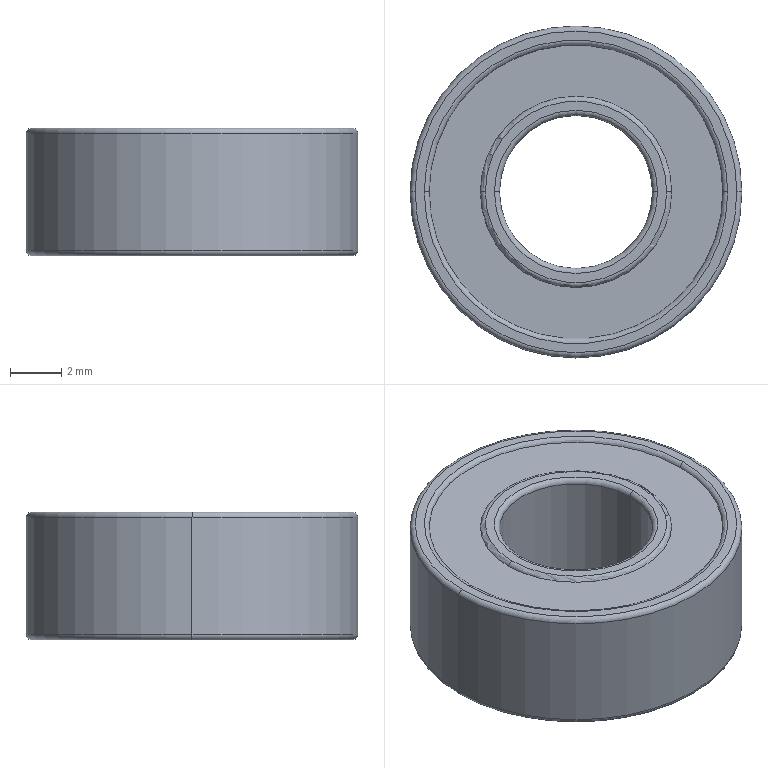Part | NX | features BREP 1 | 1 solid | 26 faces | box 13 x 13 x 5 mm | volume 502.459 mm3 | torus 16 | plane 6 | cylinder 4 | commonest cylinder face diameters 6 x2 13 x2
STEP:
#1=CARTESIAN_POINT('',(3.,0.,-0.2));
#2=VERTEX_POINT('',#1);
#3=CARTESIAN_POINT('',(3.2,0.,0.));
#4=VERTEX_POINT('',#3);
#5=CARTESIAN_POINT('',(3.2,0.,-0.2));
#6=DIRECTION('',(0.,1.,0.));
#7=DIRECTION('',(-1.,0.,0.));
#8=AXIS2_PLACEMENT_3D('',#5,#6,#7);
#9=CIRCLE('',#8,0.2);
#10=EDGE_CURVE('',#2,#4,#9,.T.);
#11=ORIENTED_EDGE('',*,*,#10,.F.);
#12=CARTESIAN_POINT('',(-3.,0.,-0.2));
#13=VERTEX_POINT('',#12);
#14=CARTESIAN_POINT('',(0.,0.,-0.2));
#15=DIRECTION('',(0.,0.,1.));
#16=DIRECTION('',(-1.,0.,0.));
#17=AXIS2_PLACEMENT_3D('',#14,#15,#16);
#18=CIRCLE('',#17,3.);
#19=EDGE_CURVE('',#13,#2,#18,.T.);
#20=ORIENTED_EDGE('',*,*,#19,.F.);
#21=CARTESIAN_POINT('',(-3.2,0.,0.));
#22=VERTEX_POINT('',#21);
#23=CARTESIAN_POINT('',(-3.2,0.,-0.2));
#24=DIRECTION('',(0.,-1.,0.));
#25=DIRECTION('',(0.,0.,-1.));
#26=AXIS2_PLACEMENT_3D('',#23,#24,#25);
#27=CIRCLE('',#26,0.2);
#28=EDGE_CURVE('',#13,#22,#27,.T.);
#29=ORIENTED_EDGE('',*,*,#28,.T.);
#30=CARTESIAN_POINT('',(0.,0.,0.));
#31=DIRECTION('',(0.,0.,-1.));
#32=DIRECTION('',(-1.,0.,0.));
#33=AXIS2_PLACEMENT_3D('',#30,#31,#32);
#34=CIRCLE('',#33,3.2);
#35=EDGE_CURVE('',#4,#22,#34,.T.);
#36=ORIENTED_EDGE('',*,*,#35,.F.);
#37=EDGE_LOOP('',(#11,#20,#29,#36));
#38=FACE_BOUND('',#37,.T.);
#39=CARTESIAN_POINT('',(0.,0.,-0.2));
#40=DIRECTION('',(0.,0.,-1.));
#41=DIRECTION('',(-1.,0.,0.));
#42=AXIS2_PLACEMENT_3D('',#39,#40,#41);
#43=TOROIDAL_SURFACE('',#42,3.2,0.2);
#44=ADVANCED_FACE('',(#38),#43,.T.);
#45=CARTESIAN_POINT('',(5.75,0.,-0.15));
#46=VERTEX_POINT('',#45);
#47=CARTESIAN_POINT('',(5.944,0.,0.));
#48=VERTEX_POINT('',#47);
#49=CARTESIAN_POINT('',(5.944,0.,-0.2));
#50=DIRECTION('',(0.,1.,0.));
#51=DIRECTION('',(-1.,0.,0.));
#52=AXIS2_PLACEMENT_3D('',#49,#50,#51);
#53=CIRCLE('',#52,0.2);
#54=EDGE_CURVE('',#46,#48,#53,.T.);
#55=ORIENTED_EDGE('',*,*,#54,.F.);
#56=CARTESIAN_POINT('',(-5.75,0.,-0.15));
#57=VERTEX_POINT('',#56);
#58=CARTESIAN_POINT('',(0.,0.,-0.15));
#59=DIRECTION('',(0.,0.,1.));
#60=DIRECTION('',(1.,0.,0.));
#61=AXIS2_PLACEMENT_3D('',#58,#59,#60);
#62=CIRCLE('',#61,5.75);
#63=EDGE_CURVE('',#57,#46,#62,.T.);
#64=ORIENTED_EDGE('',*,*,#63,.F.);
#65=CARTESIAN_POINT('',(-5.944,0.,0.));
#66=VERTEX_POINT('',#65);
#67=CARTESIAN_POINT('',(-5.944,0.,-0.2));
#68=DIRECTION('',(0.,-1.,0.));
#69=DIRECTION('',(0.,0.,-1.));
#70=AXIS2_PLACEMENT_3D('',#67,#68,#69);
#71=CIRCLE('',#70,0.2);
#72=EDGE_CURVE('',#57,#66,#71,.T.);
#73=ORIENTED_EDGE('',*,*,#72,.T.);
#74=CARTESIAN_POINT('',(0.,0.,0.));
#75=DIRECTION('',(0.,0.,-1.));
#76=DIRECTION('',(-1.,0.,0.));
#77=AXIS2_PLACEMENT_3D('',#74,#75,#76);
#78=CIRCLE('',#77,5.944);
#79=EDGE_CURVE('',#48,#66,#78,.T.);
#80=ORIENTED_EDGE('',*,*,#79,.F.);
#81=EDGE_LOOP('',(#55,#64,#73,#80));
#82=FACE_BOUND('',#81,.T.);
#83=CARTESIAN_POINT('',(0.,0.,-0.2));
#84=DIRECTION('',(0.,0.,-1.));
#85=DIRECTION('',(-1.,0.,0.));
#86=AXIS2_PLACEMENT_3D('',#83,#84,#85);
#87=TOROIDAL_SURFACE('',#86,5.944,0.2);
#88=ADVANCED_FACE('',(#82),#87,.T.);
#89=CARTESIAN_POINT('',(-3.556,0.,0.));
#90=VERTEX_POINT('',#89);
#91=CARTESIAN_POINT('',(-3.75,0.,-0.15));
#92=VERTEX_POINT('',#91);
#93=CARTESIAN_POINT('',(-3.556,0.,-0.2));
#94=DIRECTION('',(0.,1.,0.));
#95=DIRECTION('',(-1.,0.,0.));
#96=AXIS2_PLACEMENT_3D('',#93,#94,#95);
#97=CIRCLE('',#96,0.2);
#98=EDGE_CURVE('',#90,#92,#97,.F.);
#99=ORIENTED_EDGE('',*,*,#98,.T.);
#100=CARTESIAN_POINT('',(3.75,0.,-0.15));
#101=VERTEX_POINT('',#100);
#102=CARTESIAN_POINT('',(0.,0.,-0.15));
#103=DIRECTION('',(0.,0.,1.));
#104=DIRECTION('',(1.,0.,0.));
#105=AXIS2_PLACEMENT_3D('',#102,#103,#104);
#106=CIRCLE('',#105,3.75);
#107=EDGE_CURVE('',#92,#101,#106,.T.);
#108=ORIENTED_EDGE('',*,*,#107,.T.);
#109=CARTESIAN_POINT('',(3.556,0.,0.));
#110=VERTEX_POINT('',#109);
#111=CARTESIAN_POINT('',(3.556,0.,-0.2));
#112=DIRECTION('',(0.,-1.,0.));
#113=DIRECTION('',(0.,0.,-1.));
#114=AXIS2_PLACEMENT_3D('',#111,#112,#113);
#115=CIRCLE('',#114,0.2);
#116=EDGE_CURVE('',#110,#101,#115,.F.);
#117=ORIENTED_EDGE('',*,*,#116,.F.);
#118=CARTESIAN_POINT('',(0.,0.,0.));
#119=DIRECTION('',(0.,0.,1.));
#120=DIRECTION('',(-1.,0.,0.));
#121=AXIS2_PLACEMENT_3D('',#118,#119,#120);
#122=CIRCLE('',#121,3.556);
#123=EDGE_CURVE('',#90,#110,#122,.T.);
#124=ORIENTED_EDGE('',*,*,#123,.F.);
#125=EDGE_LOOP('',(#99,#108,#117,#124));
#126=FACE_BOUND('',#125,.T.);
#127=CARTESIAN_POINT('',(0.,0.,-0.2));
#128=DIRECTION('',(0.,0.,1.));
#129=DIRECTION('',(1.,0.,0.));
#130=AXIS2_PLACEMENT_3D('',#127,#128,#129);
#131=TOROIDAL_SURFACE('',#130,3.556,0.2);
#132=ADVANCED_FACE('',(#126),#131,.T.);
#133=CARTESIAN_POINT('',(6.3,0.,0.));
#134=VERTEX_POINT('',#133);
#135=CARTESIAN_POINT('',(6.5,0.,-0.2));
#136=VERTEX_POINT('',#135);
#137=CARTESIAN_POINT('',(6.3,0.,-0.2));
#138=DIRECTION('',(0.,1.,0.));
#139=DIRECTION('',(-1.,0.,0.));
#140=AXIS2_PLACEMENT_3D('',#137,#138,#139);
#141=CIRCLE('',#140,0.2);
#142=EDGE_CURVE('',#134,#136,#141,.T.);
#143=ORIENTED_EDGE('',*,*,#142,.F.);
#144=CARTESIAN_POINT('',(-6.3,0.,0.));
#145=VERTEX_POINT('',#144);
#146=CARTESIAN_POINT('',(0.,0.,0.));
#147=DIRECTION('',(0.,0.,1.));
#148=DIRECTION('',(-1.,0.,0.));
#149=AXIS2_PLACEMENT_3D('',#146,#147,#148);
#150=CIRCLE('',#149,6.3);
#151=EDGE_CURVE('',#145,#134,#150,.T.);
#152=ORIENTED_EDGE('',*,*,#151,.F.);
#153=CARTESIAN_POINT('',(-6.5,0.,-0.2));
#154=VERTEX_POINT('',#153);
#155=CARTESIAN_POINT('',(-6.3,0.,-0.2));
#156=DIRECTION('',(0.,-1.,0.));
#157=DIRECTION('',(0.,0.,-1.));
#158=AXIS2_PLACEMENT_3D('',#155,#156,#157);
#159=CIRCLE('',#158,0.2);
#160=EDGE_CURVE('',#145,#154,#159,.T.);
#161=ORIENTED_EDGE('',*,*,#160,.T.);
#162=CARTESIAN_POINT('',(0.,0.,-0.2));
#163=DIRECTION('',(0.,0.,-1.));
#164=DIRECTION('',(-1.,0.,0.));
#165=AXIS2_PLACEMENT_3D('',#162,#163,#164);
#166=CIRCLE('',#165,6.5);
#167=EDGE_CURVE('',#136,#154,#166,.T.);
#168=ORIENTED_EDGE('',*,*,#167,.F.);
#169=EDGE_LOOP('',(#143,#152,#161,#168));
#170=FACE_BOUND('',#169,.T.);
#171=CARTESIAN_POINT('',(0.,0.,-0.2));
#172=DIRECTION('',(0.,0.,-1.));
#173=DIRECTION('',(-1.,0.,0.));
#174=AXIS2_PLACEMENT_3D('',#171,#172,#173);
#175=TOROIDAL_SURFACE('',#174,6.3,0.2);
#176=ADVANCED_FACE('',(#170),#175,.T.);
#177=CARTESIAN_POINT('',(-6.5,0.,-4.8));
#178=VERTEX_POINT('',#177);
#179=CARTESIAN_POINT('',(-6.3,0.,-5.));
#180=VERTEX_POINT('',#179);
#181=CARTESIAN_POINT('',(-6.3,0.,-4.8));
#182=DIRECTION('',(0.,1.,0.));
#183=DIRECTION('',(-1.,0.,0.));
#184=AXIS2_PLACEMENT_3D('',#181,#182,#183);
#185=CIRCLE('',#184,0.2);
#186=EDGE_CURVE('',#178,#180,#185,.F.);
#187=ORIENTED_EDGE('',*,*,#186,.T.);
#188=CARTESIAN_POINT('',(6.3,0.,-5.));
#189=VERTEX_POINT('',#188);
#190=CARTESIAN_POINT('',(0.,0.,-5.));
#191=DIRECTION('',(0.,0.,-1.));
#192=DIRECTION('',(1.,0.,0.));
#193=AXIS2_PLACEMENT_3D('',#190,#191,#192);
#194=CIRCLE('',#193,6.3);
#195=EDGE_CURVE('',#189,#180,#194,.T.);
#196=ORIENTED_EDGE('',*,*,#195,.F.);
#197=CARTESIAN_POINT('',(6.5,0.,-4.8));
#198=VERTEX_POINT('',#197);
#199=CARTESIAN_POINT('',(6.3,0.,-4.8));
#200=DIRECTION('',(0.,-1.,0.));
#201=DIRECTION('',(0.,0.,-1.));
#202=AXIS2_PLACEMENT_3D('',#199,#200,#201);
#203=CIRCLE('',#202,0.2);
#204=EDGE_CURVE('',#198,#189,#203,.F.);
#205=ORIENTED_EDGE('',*,*,#204,.F.);
#206=CARTESIAN_POINT('',(0.,0.,-4.8));
#207=DIRECTION('',(0.,0.,1.));
#208=DIRECTION('',(1.,0.,0.));
#209=AXIS2_PLACEMENT_3D('',#206,#207,#208);
#210=CIRCLE('',#209,6.5);
#211=EDGE_CURVE('',#178,#198,#210,.T.);
#212=ORIENTED_EDGE('',*,*,#211,.F.);
#213=EDGE_LOOP('',(#187,#196,#205,#212));
#214=FACE_BOUND('',#213,.T.);
#215=CARTESIAN_POINT('',(0.,0.,-4.8));
#216=DIRECTION('',(0.,0.,1.));
#217=DIRECTION('',(1.,0.,0.));
#218=AXIS2_PLACEMENT_3D('',#215,#216,#217);
#219=TOROIDAL_SURFACE('',#218,6.3,0.2);
#220=ADVANCED_FACE('',(#214),#219,.T.);
#221=CARTESIAN_POINT('',(-5.944,0.,-5.));
#222=VERTEX_POINT('',#221);
#223=CARTESIAN_POINT('',(-5.75,0.,-4.85));
#224=VERTEX_POINT('',#223);
#225=CARTESIAN_POINT('',(-5.944,0.,-4.8));
#226=DIRECTION('',(0.,1.,0.));
#227=DIRECTION('',(-1.,0.,0.));
#228=AXIS2_PLACEMENT_3D('',#225,#226,#227);
#229=CIRCLE('',#228,0.2);
#230=EDGE_CURVE('',#222,#224,#229,.F.);
#231=ORIENTED_EDGE('',*,*,#230,.T.);
#232=CARTESIAN_POINT('',(5.75,0.,-4.85));
#233=VERTEX_POINT('',#232);
#234=CARTESIAN_POINT('',(0.,0.,-4.85));
#235=DIRECTION('',(0.,0.,1.));
#236=DIRECTION('',(1.,0.,0.));
#237=AXIS2_PLACEMENT_3D('',#234,#235,#236);
#238=CIRCLE('',#237,5.75);
#239=EDGE_CURVE('',#224,#233,#238,.T.);
#240=ORIENTED_EDGE('',*,*,#239,.T.);
#241=CARTESIAN_POINT('',(5.944,0.,-5.));
#242=VERTEX_POINT('',#241);
#243=CARTESIAN_POINT('',(5.944,0.,-4.8));
#244=DIRECTION('',(0.,-1.,0.));
#245=DIRECTION('',(0.,0.,-1.));
#246=AXIS2_PLACEMENT_3D('',#243,#244,#245);
#247=CIRCLE('',#246,0.2);
#248=EDGE_CURVE('',#242,#233,#247,.F.);
#249=ORIENTED_EDGE('',*,*,#248,.F.);
#250=CARTESIAN_POINT('',(0.,0.,-5.));
#251=DIRECTION('',(0.,0.,1.));
#252=DIRECTION('',(1.,0.,0.));
#253=AXIS2_PLACEMENT_3D('',#250,#251,#252);
#254=CIRCLE('',#253,5.944);
#255=EDGE_CURVE('',#222,#242,#254,.T.);
#256=ORIENTED_EDGE('',*,*,#255,.F.);
#257=EDGE_LOOP('',(#231,#240,#249,#256));
#258=FACE_BOUND('',#257,.T.);
#259=CARTESIAN_POINT('',(0.,0.,-4.8));
#260=DIRECTION('',(0.,0.,1.));
#261=DIRECTION('',(1.,0.,0.));
#262=AXIS2_PLACEMENT_3D('',#259,#260,#261);
#263=TOROIDAL_SURFACE('',#262,5.944,0.2);
#264=ADVANCED_FACE('',(#258),#263,.T.);
#265=CARTESIAN_POINT('',(3.75,0.,-4.85));
#266=VERTEX_POINT('',#265);
#267=CARTESIAN_POINT('',(3.556,0.,-5.));
#268=VERTEX_POINT('',#267);
#269=CARTESIAN_POINT('',(3.556,0.,-4.8));
#270=DIRECTION('',(0.,1.,0.));
#271=DIRECTION('',(-1.,0.,0.));
#272=AXIS2_PLACEMENT_3D('',#269,#270,#271);
#273=CIRCLE('',#272,0.2);
#274=EDGE_CURVE('',#266,#268,#273,.T.);
#275=ORIENTED_EDGE('',*,*,#274,.F.);
#276=CARTESIAN_POINT('',(-3.75,0.,-4.85));
#277=VERTEX_POINT('',#276);
#278=CARTESIAN_POINT('',(0.,0.,-4.85));
#279=DIRECTION('',(0.,0.,1.));
#280=DIRECTION('',(1.,0.,0.));
#281=AXIS2_PLACEMENT_3D('',#278,#279,#280);
#282=CIRCLE('',#281,3.75);
#283=EDGE_CURVE('',#277,#266,#282,.T.);
#284=ORIENTED_EDGE('',*,*,#283,.F.);
#285=CARTESIAN_POINT('',(-3.556,0.,-5.));
#286=VERTEX_POINT('',#285);
#287=CARTESIAN_POINT('',(-3.556,0.,-4.8));
#288=DIRECTION('',(0.,-1.,0.));
#289=DIRECTION('',(0.,0.,-1.));
#290=AXIS2_PLACEMENT_3D('',#287,#288,#289);
#291=CIRCLE('',#290,0.2);
#292=EDGE_CURVE('',#277,#286,#291,.T.);
#293=ORIENTED_EDGE('',*,*,#292,.T.);
#294=CARTESIAN_POINT('',(0.,0.,-5.));
#295=DIRECTION('',(0.,0.,-1.));
#296=DIRECTION('',(1.,0.,0.));
#297=AXIS2_PLACEMENT_3D('',#294,#295,#296);
#298=CIRCLE('',#297,3.556);
#299=EDGE_CURVE('',#268,#286,#298,.T.);
#300=ORIENTED_EDGE('',*,*,#299,.F.);
#301=EDGE_LOOP('',(#275,#284,#293,#300));
#302=FACE_BOUND('',#301,.T.);
#303=CARTESIAN_POINT('',(0.,0.,-4.8));
#304=DIRECTION('',(0.,0.,-1.));
#305=DIRECTION('',(-1.,0.,0.));
#306=AXIS2_PLACEMENT_3D('',#303,#304,#305);
#307=TOROIDAL_SURFACE('',#306,3.556,0.2);
#308=ADVANCED_FACE('',(#302),#307,.T.);
#309=CARTESIAN_POINT('',(-3.2,0.,-5.));
#310=VERTEX_POINT('',#309);
#311=CARTESIAN_POINT('',(-3.,0.,-4.8));
#312=VERTEX_POINT('',#311);
#313=CARTESIAN_POINT('',(-3.2,0.,-4.8));
#314=DIRECTION('',(0.,1.,0.));
#315=DIRECTION('',(-1.,0.,0.));
#316=AXIS2_PLACEMENT_3D('',#313,#314,#315);
#317=CIRCLE('',#316,0.2);
#318=EDGE_CURVE('',#310,#312,#317,.F.);
#319=ORIENTED_EDGE('',*,*,#318,.T.);
#320=CARTESIAN_POINT('',(3.,0.,-4.8));
#321=VERTEX_POINT('',#320);
#322=CARTESIAN_POINT('',(0.,0.,-4.8));
#323=DIRECTION('',(0.,0.,-1.));
#324=DIRECTION('',(1.,0.,0.));
#325=AXIS2_PLACEMENT_3D('',#322,#323,#324);
#326=CIRCLE('',#325,3.);
#327=EDGE_CURVE('',#321,#312,#326,.T.);
#328=ORIENTED_EDGE('',*,*,#327,.F.);
#329=CARTESIAN_POINT('',(3.2,0.,-5.));
#330=VERTEX_POINT('',#329);
#331=CARTESIAN_POINT('',(3.2,0.,-4.8));
#332=DIRECTION('',(0.,-1.,0.));
#333=DIRECTION('',(0.,0.,-1.));
#334=AXIS2_PLACEMENT_3D('',#331,#332,#333);
#335=CIRCLE('',#334,0.2);
#336=EDGE_CURVE('',#330,#321,#335,.F.);
#337=ORIENTED_EDGE('',*,*,#336,.F.);
#338=CARTESIAN_POINT('',(0.,0.,-5.));
#339=DIRECTION('',(0.,0.,1.));
#340=DIRECTION('',(1.,0.,0.));
#341=AXIS2_PLACEMENT_3D('',#338,#339,#340);
#342=CIRCLE('',#341,3.2);
#343=EDGE_CURVE('',#310,#330,#342,.T.);
#344=ORIENTED_EDGE('',*,*,#343,.F.);
#345=EDGE_LOOP('',(#319,#328,#337,#344));
#346=FACE_BOUND('',#345,.T.);
#347=CARTESIAN_POINT('',(0.,0.,-4.8));
#348=DIRECTION('',(0.,0.,1.));
#349=DIRECTION('',(1.,0.,0.));
#350=AXIS2_PLACEMENT_3D('',#347,#348,#349);
#351=TOROIDAL_SURFACE('',#350,3.2,0.2);
#352=ADVANCED_FACE('',(#346),#351,.T.);
#353=ORIENTED_EDGE('',*,*,#63,.T.);
#354=CARTESIAN_POINT('',(0.,0.,-0.15));
#355=DIRECTION('',(0.,0.,1.));
#356=DIRECTION('',(1.,0.,0.));
#357=AXIS2_PLACEMENT_3D('',#354,#355,#356);
#358=CIRCLE('',#357,5.75);
#359=EDGE_CURVE('',#46,#57,#358,.T.);
#360=ORIENTED_EDGE('',*,*,#359,.T.);
#361=EDGE_LOOP('',(#353,#360));
#362=FACE_BOUND('',#361,.T.);
#363=CARTESIAN_POINT('',(0.,0.,-0.15));
#364=DIRECTION('',(0.,0.,1.));
#365=DIRECTION('',(1.,0.,0.));
#366=AXIS2_PLACEMENT_3D('',#363,#364,#365);
#367=CIRCLE('',#366,3.75);
#368=EDGE_CURVE('',#101,#92,#367,.T.);
#369=ORIENTED_EDGE('',*,*,#368,.F.);
#370=ORIENTED_EDGE('',*,*,#107,.F.);
#371=EDGE_LOOP('',(#369,#370));
#372=FACE_BOUND('',#371,.T.);
#373=CARTESIAN_POINT('',(-5.75,0.,-0.15));
#374=DIRECTION('',(0.,0.,-1.));
#375=DIRECTION('',(-1.,0.,0.));
#376=AXIS2_PLACEMENT_3D('',#373,#374,#375);
#377=PLANE('',#376);
#378=ADVANCED_FACE('',(#362,#372),#377,.F.);
#379=CARTESIAN_POINT('',(0.,0.,0.));
#380=DIRECTION('',(0.,0.,-1.));
#381=DIRECTION('',(-1.,0.,0.));
#382=AXIS2_PLACEMENT_3D('',#379,#380,#381);
#383=CIRCLE('',#382,5.944);
#384=EDGE_CURVE('',#66,#48,#383,.T.);
#385=ORIENTED_EDGE('',*,*,#384,.T.);
#386=ORIENTED_EDGE('',*,*,#79,.T.);
#387=EDGE_LOOP('',(#385,#386));
#388=FACE_BOUND('',#387,.T.);
#389=ORIENTED_EDGE('',*,*,#151,.T.);
#390=CARTESIAN_POINT('',(0.,0.,0.));
#391=DIRECTION('',(0.,0.,1.));
#392=DIRECTION('',(-1.,0.,0.));
#393=AXIS2_PLACEMENT_3D('',#390,#391,#392);
#394=CIRCLE('',#393,6.3);
#395=EDGE_CURVE('',#134,#145,#394,.T.);
#396=ORIENTED_EDGE('',*,*,#395,.T.);
#397=EDGE_LOOP('',(#389,#396));
#398=FACE_BOUND('',#397,.T.);
#399=CARTESIAN_POINT('',(-6.5,0.,0.));
#400=DIRECTION('',(0.,0.,-1.));
#401=DIRECTION('',(-1.,0.,0.));
#402=AXIS2_PLACEMENT_3D('',#399,#400,#401);
#403=PLANE('',#402);
#404=ADVANCED_FACE('',(#388,#398),#403,.F.);
#405=CARTESIAN_POINT('',(-6.5,0.,0.));
#406=DIRECTION('',(0.,0.,1.));
#407=VECTOR('',#406,1000.);
#408=LINE('',#405,#407);
#409=EDGE_CURVE('',#154,#178,#408,.F.);
#410=ORIENTED_EDGE('',*,*,#409,.T.);
#411=ORIENTED_EDGE('',*,*,#211,.T.);
#412=CARTESIAN_POINT('',(6.5,0.,0.));
#413=DIRECTION('',(0.,0.,1.));
#414=VECTOR('',#413,1000.);
#415=LINE('',#412,#414);
#416=EDGE_CURVE('',#136,#198,#415,.F.);
#417=ORIENTED_EDGE('',*,*,#416,.F.);
#418=ORIENTED_EDGE('',*,*,#167,.T.);
#419=EDGE_LOOP('',(#410,#411,#417,#418));
#420=FACE_BOUND('',#419,.T.);
#421=CARTESIAN_POINT('',(0.,0.,0.));
#422=DIRECTION('',(0.,0.,1.));
#423=DIRECTION('',(1.,0.,0.));
#424=AXIS2_PLACEMENT_3D('',#421,#422,#423);
#425=CYLINDRICAL_SURFACE('',#424,6.5);
#426=ADVANCED_FACE('',(#420),#425,.T.);
#427=ORIENTED_EDGE('',*,*,#195,.T.);
#428=CARTESIAN_POINT('',(0.,0.,-5.));
#429=DIRECTION('',(0.,0.,-1.));
#430=DIRECTION('',(1.,0.,0.));
#431=AXIS2_PLACEMENT_3D('',#428,#429,#430);
#432=CIRCLE('',#431,6.3);
#433=EDGE_CURVE('',#180,#189,#432,.T.);
#434=ORIENTED_EDGE('',*,*,#433,.T.);
#435=EDGE_LOOP('',(#427,#434));
#436=FACE_BOUND('',#435,.T.);
#437=CARTESIAN_POINT('',(0.,0.,-5.));
#438=DIRECTION('',(0.,0.,1.));
#439=DIRECTION('',(1.,0.,0.));
#440=AXIS2_PLACEMENT_3D('',#437,#438,#439);
#441=CIRCLE('',#440,5.944);
#442=EDGE_CURVE('',#242,#222,#441,.T.);
#443=ORIENTED_EDGE('',*,*,#442,.T.);
#444=ORIENTED_EDGE('',*,*,#255,.T.);
#445=EDGE_LOOP('',(#443,#444));
#446=FACE_BOUND('',#445,.T.);
#447=CARTESIAN_POINT('',(-5.75,0.,-5.));
#448=DIRECTION('',(0.,0.,1.));
#449=DIRECTION('',(1.,0.,0.));
#450=AXIS2_PLACEMENT_3D('',#447,#448,#449);
#451=PLANE('',#450);
#452=ADVANCED_FACE('',(#436,#446),#451,.F.);
#453=ORIENTED_EDGE('',*,*,#283,.T.);
#454=CARTESIAN_POINT('',(0.,0.,-4.85));
#455=DIRECTION('',(0.,0.,1.));
#456=DIRECTION('',(1.,0.,0.));
#457=AXIS2_PLACEMENT_3D('',#454,#455,#456);
#458=CIRCLE('',#457,3.75);
#459=EDGE_CURVE('',#266,#277,#458,.T.);
#460=ORIENTED_EDGE('',*,*,#459,.T.);
#461=EDGE_LOOP('',(#453,#460));
#462=FACE_BOUND('',#461,.T.);
#463=CARTESIAN_POINT('',(0.,0.,-4.85));
#464=DIRECTION('',(0.,0.,1.));
#465=DIRECTION('',(1.,0.,0.));
#466=AXIS2_PLACEMENT_3D('',#463,#464,#465);
#467=CIRCLE('',#466,5.75);
#468=EDGE_CURVE('',#233,#224,#467,.T.);
#469=ORIENTED_EDGE('',*,*,#468,.F.);
#470=ORIENTED_EDGE('',*,*,#239,.F.);
#471=EDGE_LOOP('',(#469,#470));
#472=FACE_BOUND('',#471,.T.);
#473=CARTESIAN_POINT('',(-3.75,0.,-4.85));
#474=DIRECTION('',(0.,0.,1.));
#475=DIRECTION('',(1.,0.,0.));
#476=AXIS2_PLACEMENT_3D('',#473,#474,#475);
#477=PLANE('',#476);
#478=ADVANCED_FACE('',(#462,#472),#477,.F.);
#479=CARTESIAN_POINT('',(0.,0.,-5.));
#480=DIRECTION('',(0.,0.,-1.));
#481=DIRECTION('',(1.,0.,0.));
#482=AXIS2_PLACEMENT_3D('',#479,#480,#481);
#483=CIRCLE('',#482,3.556);
#484=EDGE_CURVE('',#286,#268,#483,.T.);
#485=ORIENTED_EDGE('',*,*,#484,.T.);
#486=ORIENTED_EDGE('',*,*,#299,.T.);
#487=EDGE_LOOP('',(#485,#486));
#488=FACE_BOUND('',#487,.T.);
#489=CARTESIAN_POINT('',(0.,0.,-5.));
#490=DIRECTION('',(0.,0.,1.));
#491=DIRECTION('',(1.,0.,0.));
#492=AXIS2_PLACEMENT_3D('',#489,#490,#491);
#493=CIRCLE('',#492,3.2);
#494=EDGE_CURVE('',#330,#310,#493,.T.);
#495=ORIENTED_EDGE('',*,*,#494,.T.);
#496=ORIENTED_EDGE('',*,*,#343,.T.);
#497=EDGE_LOOP('',(#495,#496));
#498=FACE_BOUND('',#497,.T.);
#499=CARTESIAN_POINT('',(-3.,0.,-5.));
#500=DIRECTION('',(0.,0.,1.));
#501=DIRECTION('',(1.,0.,0.));
#502=AXIS2_PLACEMENT_3D('',#499,#500,#501);
#503=PLANE('',#502);
#504=ADVANCED_FACE('',(#488,#498),#503,.F.);
#505=CARTESIAN_POINT('',(-3.,0.,0.));
#506=DIRECTION('',(0.,0.,1.));
#507=VECTOR('',#506,1000.);
#508=LINE('',#505,#507);
#509=EDGE_CURVE('',#13,#312,#508,.F.);
#510=ORIENTED_EDGE('',*,*,#509,.T.);
#511=CARTESIAN_POINT('',(0.,0.,-4.8));
#512=DIRECTION('',(0.,0.,-1.));
#513=DIRECTION('',(1.,0.,0.));
#514=AXIS2_PLACEMENT_3D('',#511,#512,#513);
#515=CIRCLE('',#514,3.);
#516=EDGE_CURVE('',#312,#321,#515,.T.);
#517=ORIENTED_EDGE('',*,*,#516,.T.);
#518=CARTESIAN_POINT('',(3.,0.,0.));
#519=DIRECTION('',(0.,0.,1.));
#520=VECTOR('',#519,1000.);
#521=LINE('',#518,#520);
#522=EDGE_CURVE('',#2,#321,#521,.F.);
#523=ORIENTED_EDGE('',*,*,#522,.F.);
#524=CARTESIAN_POINT('',(0.,0.,-0.2));
#525=DIRECTION('',(0.,0.,1.));
#526=DIRECTION('',(-1.,0.,0.));
#527=AXIS2_PLACEMENT_3D('',#524,#525,#526);
#528=CIRCLE('',#527,3.);
#529=EDGE_CURVE('',#2,#13,#528,.T.);
#530=ORIENTED_EDGE('',*,*,#529,.T.);
#531=EDGE_LOOP('',(#510,#517,#523,#530));
#532=FACE_BOUND('',#531,.T.);
#533=CARTESIAN_POINT('',(0.,0.,0.));
#534=DIRECTION('',(0.,0.,1.));
#535=DIRECTION('',(1.,0.,0.));
#536=AXIS2_PLACEMENT_3D('',#533,#534,#535);
#537=CYLINDRICAL_SURFACE('',#536,3.);
#538=ADVANCED_FACE('',(#532),#537,.F.);
#539=CARTESIAN_POINT('',(0.,0.,0.));
#540=DIRECTION('',(0.,0.,-1.));
#541=DIRECTION('',(-1.,0.,0.));
#542=AXIS2_PLACEMENT_3D('',#539,#540,#541);
#543=CIRCLE('',#542,3.2);
#544=EDGE_CURVE('',#22,#4,#543,.T.);
#545=ORIENTED_EDGE('',*,*,#544,.T.);
#546=ORIENTED_EDGE('',*,*,#35,.T.);
#547=EDGE_LOOP('',(#545,#546));
#548=FACE_BOUND('',#547,.T.);
#549=CARTESIAN_POINT('',(0.,0.,0.));
#550=DIRECTION('',(0.,0.,1.));
#551=DIRECTION('',(-1.,0.,0.));
#552=AXIS2_PLACEMENT_3D('',#549,#550,#551);
#553=CIRCLE('',#552,3.556);
#554=EDGE_CURVE('',#110,#90,#553,.T.);
#555=ORIENTED_EDGE('',*,*,#554,.T.);
#556=ORIENTED_EDGE('',*,*,#123,.T.);
#557=EDGE_LOOP('',(#555,#556));
#558=FACE_BOUND('',#557,.T.);
#559=CARTESIAN_POINT('',(-3.75,0.,0.));
#560=DIRECTION('',(0.,0.,-1.));
#561=DIRECTION('',(-1.,0.,0.));
#562=AXIS2_PLACEMENT_3D('',#559,#560,#561);
#563=PLANE('',#562);
#564=ADVANCED_FACE('',(#548,#558),#563,.F.);
#565=ORIENTED_EDGE('',*,*,#327,.T.);
#566=ORIENTED_EDGE('',*,*,#509,.F.);
#567=ORIENTED_EDGE('',*,*,#19,.T.);
#568=ORIENTED_EDGE('',*,*,#522,.T.);
#569=EDGE_LOOP('',(#565,#566,#567,#568));
#570=FACE_BOUND('',#569,.T.);
#571=CARTESIAN_POINT('',(0.,0.,0.));
#572=DIRECTION('',(0.,0.,1.));
#573=DIRECTION('',(1.,0.,0.));
#574=AXIS2_PLACEMENT_3D('',#571,#572,#573);
#575=CYLINDRICAL_SURFACE('',#574,3.);
#576=ADVANCED_FACE('',(#570),#575,.F.);
#577=CARTESIAN_POINT('',(0.,0.,-4.8));
#578=DIRECTION('',(0.,0.,1.));
#579=DIRECTION('',(1.,0.,0.));
#580=AXIS2_PLACEMENT_3D('',#577,#578,#579);
#581=CIRCLE('',#580,6.5);
#582=EDGE_CURVE('',#198,#178,#581,.T.);
#583=ORIENTED_EDGE('',*,*,#582,.T.);
#584=ORIENTED_EDGE('',*,*,#409,.F.);
#585=CARTESIAN_POINT('',(0.,0.,-0.2));
#586=DIRECTION('',(0.,0.,-1.));
#587=DIRECTION('',(-1.,0.,0.));
#588=AXIS2_PLACEMENT_3D('',#585,#586,#587);
#589=CIRCLE('',#588,6.5);
#590=EDGE_CURVE('',#154,#136,#589,.T.);
#591=ORIENTED_EDGE('',*,*,#590,.T.);
#592=ORIENTED_EDGE('',*,*,#416,.T.);
#593=EDGE_LOOP('',(#583,#584,#591,#592));
#594=FACE_BOUND('',#593,.T.);
#595=CARTESIAN_POINT('',(0.,0.,0.));
#596=DIRECTION('',(0.,0.,1.));
#597=DIRECTION('',(1.,0.,0.));
#598=AXIS2_PLACEMENT_3D('',#595,#596,#597);
#599=CYLINDRICAL_SURFACE('',#598,6.5);
#600=ADVANCED_FACE('',(#594),#599,.T.);
#601=ORIENTED_EDGE('',*,*,#516,.F.);
#602=ORIENTED_EDGE('',*,*,#318,.F.);
#603=ORIENTED_EDGE('',*,*,#494,.F.);
#604=ORIENTED_EDGE('',*,*,#336,.T.);
#605=EDGE_LOOP('',(#601,#602,#603,#604));
#606=FACE_BOUND('',#605,.T.);
#607=CARTESIAN_POINT('',(0.,0.,-4.8));
#608=DIRECTION('',(0.,0.,1.));
#609=DIRECTION('',(1.,0.,0.));
#610=AXIS2_PLACEMENT_3D('',#607,#608,#609);
#611=TOROIDAL_SURFACE('',#610,3.2,0.2);
#612=ADVANCED_FACE('',(#606),#611,.T.);
#613=ORIENTED_EDGE('',*,*,#459,.F.);
#614=ORIENTED_EDGE('',*,*,#274,.T.);
#615=ORIENTED_EDGE('',*,*,#484,.F.);
#616=ORIENTED_EDGE('',*,*,#292,.F.);
#617=EDGE_LOOP('',(#613,#614,#615,#616));
#618=FACE_BOUND('',#617,.T.);
#619=CARTESIAN_POINT('',(0.,0.,-4.8));
#620=DIRECTION('',(0.,0.,-1.));
#621=DIRECTION('',(-1.,0.,0.));
#622=AXIS2_PLACEMENT_3D('',#619,#620,#621);
#623=TOROIDAL_SURFACE('',#622,3.556,0.2);
#624=ADVANCED_FACE('',(#618),#623,.T.);
#625=ORIENTED_EDGE('',*,*,#468,.T.);
#626=ORIENTED_EDGE('',*,*,#230,.F.);
#627=ORIENTED_EDGE('',*,*,#442,.F.);
#628=ORIENTED_EDGE('',*,*,#248,.T.);
#629=EDGE_LOOP('',(#625,#626,#627,#628));
#630=FACE_BOUND('',#629,.T.);
#631=CARTESIAN_POINT('',(0.,0.,-4.8));
#632=DIRECTION('',(0.,0.,1.));
#633=DIRECTION('',(1.,0.,0.));
#634=AXIS2_PLACEMENT_3D('',#631,#632,#633);
#635=TOROIDAL_SURFACE('',#634,5.944,0.2);
#636=ADVANCED_FACE('',(#630),#635,.T.);
#637=ORIENTED_EDGE('',*,*,#433,.F.);
#638=ORIENTED_EDGE('',*,*,#186,.F.);
#639=ORIENTED_EDGE('',*,*,#582,.F.);
#640=ORIENTED_EDGE('',*,*,#204,.T.);
#641=EDGE_LOOP('',(#637,#638,#639,#640));
#642=FACE_BOUND('',#641,.T.);
#643=CARTESIAN_POINT('',(0.,0.,-4.8));
#644=DIRECTION('',(0.,0.,1.));
#645=DIRECTION('',(1.,0.,0.));
#646=AXIS2_PLACEMENT_3D('',#643,#644,#645);
#647=TOROIDAL_SURFACE('',#646,6.3,0.2);
#648=ADVANCED_FACE('',(#642),#647,.T.);
#649=ORIENTED_EDGE('',*,*,#395,.F.);
#650=ORIENTED_EDGE('',*,*,#142,.T.);
#651=ORIENTED_EDGE('',*,*,#590,.F.);
#652=ORIENTED_EDGE('',*,*,#160,.F.);
#653=EDGE_LOOP('',(#649,#650,#651,#652));
#654=FACE_BOUND('',#653,.T.);
#655=CARTESIAN_POINT('',(0.,0.,-0.2));
#656=DIRECTION('',(0.,0.,-1.));
#657=DIRECTION('',(-1.,0.,0.));
#658=AXIS2_PLACEMENT_3D('',#655,#656,#657);
#659=TOROIDAL_SURFACE('',#658,6.3,0.2);
#660=ADVANCED_FACE('',(#654),#659,.T.);
#661=ORIENTED_EDGE('',*,*,#368,.T.);
#662=ORIENTED_EDGE('',*,*,#98,.F.);
#663=ORIENTED_EDGE('',*,*,#554,.F.);
#664=ORIENTED_EDGE('',*,*,#116,.T.);
#665=EDGE_LOOP('',(#661,#662,#663,#664));
#666=FACE_BOUND('',#665,.T.);
#667=CARTESIAN_POINT('',(0.,0.,-0.2));
#668=DIRECTION('',(0.,0.,1.));
#669=DIRECTION('',(1.,0.,0.));
#670=AXIS2_PLACEMENT_3D('',#667,#668,#669);
#671=TOROIDAL_SURFACE('',#670,3.556,0.2);
#672=ADVANCED_FACE('',(#666),#671,.T.);
#673=ORIENTED_EDGE('',*,*,#359,.F.);
#674=ORIENTED_EDGE('',*,*,#54,.T.);
#675=ORIENTED_EDGE('',*,*,#384,.F.);
#676=ORIENTED_EDGE('',*,*,#72,.F.);
#677=EDGE_LOOP('',(#673,#674,#675,#676));
#678=FACE_BOUND('',#677,.T.);
#679=CARTESIAN_POINT('',(0.,0.,-0.2));
#680=DIRECTION('',(0.,0.,-1.));
#681=DIRECTION('',(-1.,0.,0.));
#682=AXIS2_PLACEMENT_3D('',#679,#680,#681);
#683=TOROIDAL_SURFACE('',#682,5.944,0.2);
#684=ADVANCED_FACE('',(#678),#683,.T.);
#685=ORIENTED_EDGE('',*,*,#529,.F.);
#686=ORIENTED_EDGE('',*,*,#10,.T.);
#687=ORIENTED_EDGE('',*,*,#544,.F.);
#688=ORIENTED_EDGE('',*,*,#28,.F.);
#689=EDGE_LOOP('',(#685,#686,#687,#688));
#690=FACE_BOUND('',#689,.T.);
#691=CARTESIAN_POINT('',(0.,0.,-0.2));
#692=DIRECTION('',(0.,0.,-1.));
#693=DIRECTION('',(-1.,0.,0.));
#694=AXIS2_PLACEMENT_3D('',#691,#692,#693);
#695=TOROIDAL_SURFACE('',#694,3.2,0.2);
#696=ADVANCED_FACE('',(#690),#695,.T.);
#697=CLOSED_SHELL('',(#44,#88,#132,#176,#220,#264,#308,#352,#378,#404,#426,#452,#478,#504,#538,#564,#576,#600,#612,#624,#636,#648,#660,#672,#684,#696));
#698=MANIFOLD_SOLID_BREP('',#697);
#699=(LENGTH_UNIT()NAMED_UNIT(*)SI_UNIT(.MILLI.,.METRE.));
#700=UNCERTAINTY_MEASURE_WITH_UNIT(LENGTH_MEASURE(0.00001),#699,'','');
#701=(NAMED_UNIT(*)PLANE_ANGLE_UNIT()SI_UNIT($,.RADIAN.));
#702=(NAMED_UNIT(*)SI_UNIT($,.STERADIAN.)SOLID_ANGLE_UNIT());
#703=(GEOMETRIC_REPRESENTATION_CONTEXT(3)GLOBAL_UNCERTAINTY_ASSIGNED_CONTEXT((#700))GLOBAL_UNIT_ASSIGNED_CONTEXT((#699,#701,#702))REPRESENTATION_CONTEXT('',''));
#704=ADVANCED_BREP_SHAPE_REPRESENTATION('',(#698),#703);